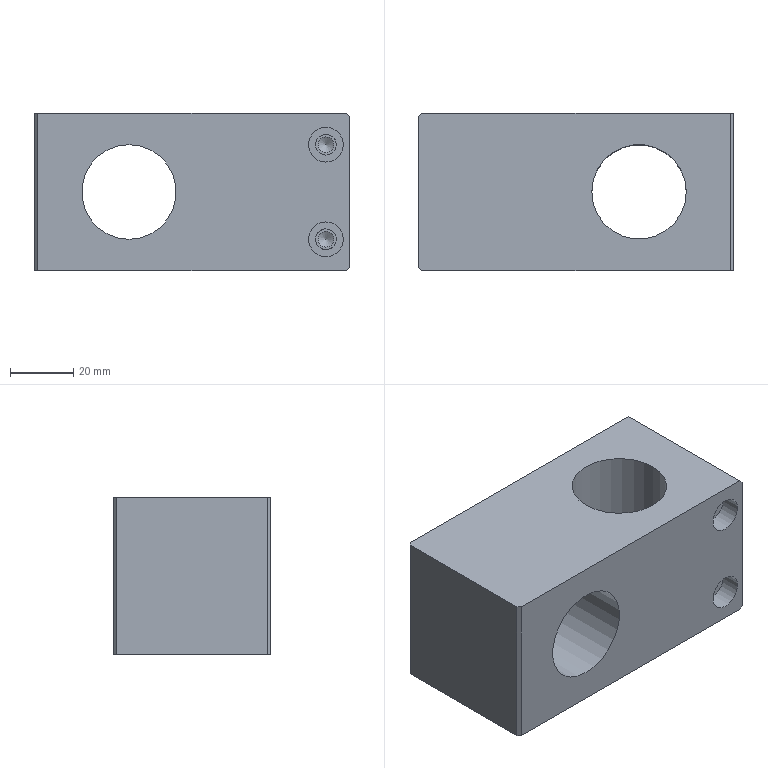CAM job | NX | 3+2 milling, drilling | part box 100 x 50 x 50 mm | stock box 105 x 55 x 55 mm
Tools:
number,name,description,diameter,corner_radius,flute_length,length,flutes
4,D4,平底铣刀-粗,4.0,0.0,25.0,75.0,2
6,D6,平底铣刀-粗,6.0,0.0,25.0,75.0,2
9,D10,平底铣刀-粗,10.0,0.0,35.0,75.0,2
7,D6-J,平底铣刀-精,6.0,0.0,25.0,75.0,2
10,D10-J,平底铣刀-精,10.0,0.0,35.0,75.0,2
1,D80R0.8飞刀,圆鼻刀-粗,80.0,0.8,50.0,75.0,2
2,D6倒角刀,倒角刀,6.0,0.0,3.0,25.0,2
15,ZT5,钻头,5.0,0.0,35.0,50.0,2
17,ZT12,钻头,12.0,0.0,35.0,50.0,2
Operations:
program,operation,operation_type,tool,method,geometry_group,spindle_rpm,surface_speed,feed_per_tooth,feed_cut,feed_plunge,cut_length_mm,path_length_mm,cut_time_min,machine_time_min
C,通用打点-深0.8_2,Operation,D6倒角刀,NONE,W-C,8000.0,150.796,0.0312,500.0,90.0,3.6,78.217,0.0072,0.0147
C,打点0.8,Operation,D6倒角刀,METHOD,W-C,8000.0,150.796,0.0312,500.0,0.0,1.8,43.6,0.0036,0.0078
C,三段孔-G83钻孔_2,Operation,ZT5,NONE,W-C,3000.0,47.124,0.0333,200.0,90.0,88.004,247.025,0.44,0.4559
C,三段孔-铣孔开粗1_2,CylinderMilling,D6,NONE,W-C,8000.0,150.796,0.075,1200.0,100.0,471.274,593.074,0.3927,0.4049
C,三段孔-铣孔开粗2_2,CylinderMilling,D4,NONE,W-C,8000.0,100.531,0.0312,500.0,100.0,866.831,1041.631,1.734,1.751
C,三段孔-铣孔精光1_2,CylinderMilling,D6-J,精光步距切深关,W-C,8000.0,150.796,0.0312,500.0,100.0,92.528,214.327,0.1851,0.1972
C,通孔-10-12.5,Operation,ZT12,NONE,W-C,1500.0,141.372,0.1,300.0,90.0,56.605,153.21,0.1887,0.1983
C,底壁铣螺旋开粗-中_COPY_COPY,VolumeBased25DMillingOperation,D10,分层开粗-切深K-步距G,W-C,5000.0,157.08,0.2,2000.0,100.0,5370.252,5458.752,2.685,2.694
C,铣倒角_3,PlanarMilling,D6倒角刀,METHOD,W-C,8000.0,150.796,0.05,800.0,100.0,81.168,187.168,0.1015,0.1121
C,铣倒角_4,PlanarMilling,D6倒角刀,METHOD,W-C,8000.0,150.796,0.05,800.0,100.0,100.274,141.274,0.1253,0.1294
C,底壁铣精光侧面-中_COPY_COPY,VolumeBased25DMillingOperation,D10-J,侧刃精光-切深K-步距G,W-C,4000.0,125.664,0.125,1000.0,100.0,430.041,550.82,0.43,0.4421
B,顶面_COPY,FaceMilling,D80R0.8飞刀,侧刃精光-切深K-步距G,W-B,5000.0,1256.637,0.1,1000.0,100.0,1940.0,3712.26,1.94,2.117
B,顶面_COPY_COPY,FaceMilling,D80R0.8飞刀,侧刃精光-切深K-步距G,W-B,5000.0,1256.637,0.1,1000.0,100.0,194.0,230.0,0.194,0.1976
B,C0.3平面去毛刺6X45L__COPY,SurfaceContour,D6倒角刀,爬面_倒角-切深0-步距G,W-B,8000.0,150.796,0.0938,1500.0,90.0,346.376,436.422,0.2312,0.2402
B,底壁铣倒角_COPY_1,VolumeBased25DMillingOperation,D6倒角刀,爬面_倒角-切深0-步距G,W-B,6500.0,122.519,0.1154,1500.0,100.0,58.801,99.201,0.0392,0.0432
A,顶面,FaceMilling,D80R0.8飞刀,侧刃精光-切深K-步距G,W-A,5000.0,1256.637,0.1,1000.0,100.0,194.0,230.0,0.194,0.1976
A,外形粗_2,VolumeBased25DMillingOperation,D10,METHOD,W-A,6000.0,188.496,0.4167,5000.0,80.0,21508.285,21597.085,4.302,4.311
A,通用打点-深0.8,Operation,D6倒角刀,NONE,W-A,8000.0,150.796,0.0312,500.0,90.0,5.4,147.099,0.0108,0.025
A,三段孔-G83钻孔,Operation,ZT5,NONE,W-A,3000.0,47.124,0.0333,200.0,90.0,88.004,247.025,0.44,0.4559
A,通孔-12.5-25,Operation,ZT12,NONE,W-A,800.0,30.159,0.1875,300.0,90.0,59.0,158.0,0.1967,0.2066
A,底壁铣螺旋开粗-中_COPY,VolumeBased25DMillingOperation,D10,分层开粗-切深K-步距G,W-A,5000.0,157.08,0.2,2000.0,100.0,5370.252,5458.752,2.685,2.694
A,三段孔-铣孔开粗1_1,CylinderMilling,D6,NONE,W-A,8000.0,150.796,0.075,1200.0,100.0,471.274,593.074,0.3927,0.4049
A,三段孔-铣孔开粗2_1,CylinderMilling,D4,NONE,W-A,8000.0,100.531,0.0375,600.0,100.0,698.819,873.619,1.165,1.182
A,三段孔-铣孔精光1_1,CylinderMilling,D6-J,精光步距切深关,W-A,8000.0,150.796,0.0312,500.0,100.0,92.528,214.327,0.1851,0.1972
A,仅选体,SurfaceContour,D6倒角刀,METHOD,W-A,8000.0,150.796,0.1875,3000.0,100.0,355.991,474.997,0.1187,0.1306
A,铣倒角_2,PlanarMilling,D6倒角刀,METHOD,W-A,8000.0,150.796,0.0625,1000.0,100.0,97.133,139.133,0.0971,0.1013
A,底壁铣倒角_COPY,VolumeBased25DMillingOperation,D6倒角刀,爬面_倒角-切深0-步距G,W-A,6500.0,122.519,0.1154,1500.0,100.0,58.801,99.201,0.0392,0.0432
A,外形半精_2,VolumeBased25DMillingOperation,D10-J,METHOD,W-A,5000.0,157.08,0.1,1000.0,100.0,1005.607,1328.837,1.006,1.038
A,铣倒角_1,PlanarMilling,D6倒角刀,METHOD,W-A,8000.0,150.796,0.05,800.0,100.0,81.168,193.762,0.1015,0.1127
A,底壁铣精光侧面-中_COPY,VolumeBased25DMillingOperation,D10-J,侧刃精光-切深K-步距G,W-A,4000.0,125.664,0.125,1000.0,100.0,430.041,551.22,0.43,0.4422